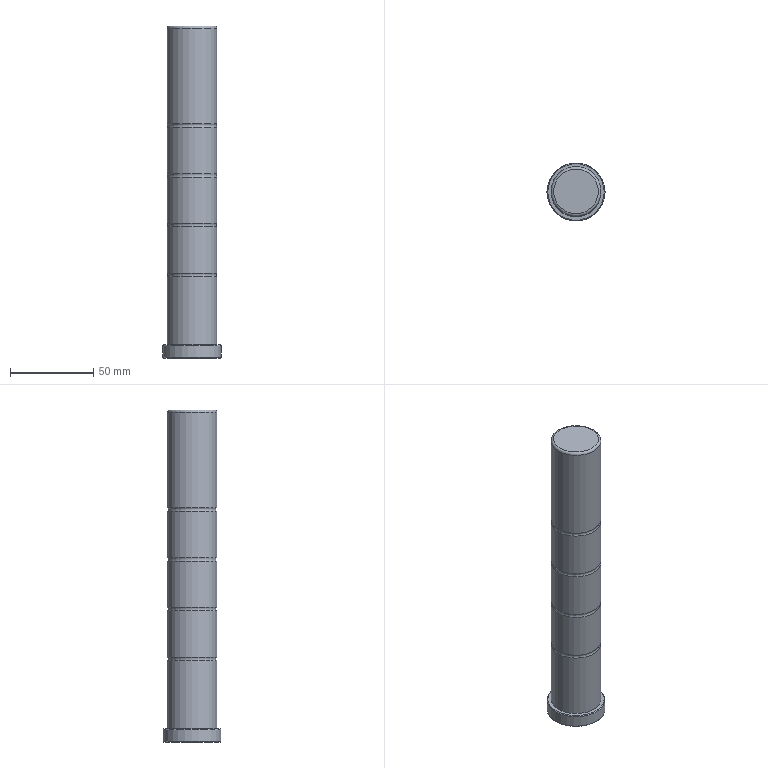Part | NX | features 模具.stp<1>[47] 2 | 1 solid | 24 faces | box 35 x 35 x 200 mm | volume 140384 mm3 | cylinder 9 | plane 7 | torus 5 | cone 3 | commonest cylinder face diameters 30 x5 10.5 x1 11.7 x1 12 x1 35 x1
STEP:
#1=CARTESIAN_POINT('',(160.,-265.,-252.505));
#2=VERTEX_POINT('',#1);
#3=VERTEX_LOOP('',#2);
#4=FACE_BOUND('',#3,.T.);
#5=CARTESIAN_POINT('',(165.25,-265.,-255.536));
#6=VERTEX_POINT('',#5);
#7=CARTESIAN_POINT('',(160.,-265.,-255.536));
#8=DIRECTION('',(0.,0.,1.));
#9=DIRECTION('',(1.,0.,0.));
#10=AXIS2_PLACEMENT_3D('',#7,#8,#9);
#11=CIRCLE('',#10,5.25);
#12=EDGE_CURVE('',#6,#6,#11,.T.);
#13=ORIENTED_EDGE('',*,*,#12,.F.);
#14=EDGE_LOOP('',(#13));
#15=FACE_BOUND('',#14,.T.);
#16=CARTESIAN_POINT('',(160.,-265.,-253.505));
#17=DIRECTION('',(0.,0.,-1.));
#18=DIRECTION('',(1.,0.,0.));
#19=AXIS2_PLACEMENT_3D('',#16,#17,#18);
#20=CONICAL_SURFACE('',#19,1.732,1.047);
#21=ADVANCED_FACE('',(#4,#15),#20,.F.);
#22=CARTESIAN_POINT('',(165.25,-265.,-261.5));
#23=VERTEX_POINT('',#22);
#24=CARTESIAN_POINT('',(165.25,-265.,-262.5));
#25=VERTEX_POINT('',#24);
#26=CARTESIAN_POINT('',(165.25,-265.,-255.536));
#27=DIRECTION('',(0.,0.,-1.));
#28=VECTOR('',#27,1000.);
#29=LINE('',#26,#28);
#30=EDGE_CURVE('',#23,#25,#29,.T.);
#31=ORIENTED_EDGE('',*,*,#30,.T.);
#32=CARTESIAN_POINT('',(160.,-270.25,-262.5));
#33=VERTEX_POINT('',#32);
#34=CARTESIAN_POINT('',(160.,-265.,-262.5));
#35=DIRECTION('',(0.,0.,1.));
#36=DIRECTION('',(0.,-1.,0.));
#37=AXIS2_PLACEMENT_3D('',#34,#35,#36);
#38=CIRCLE('',#37,5.25);
#39=EDGE_CURVE('',#25,#33,#38,.T.);
#40=ORIENTED_EDGE('',*,*,#39,.T.);
#41=CARTESIAN_POINT('',(160.,-270.25,-261.5));
#42=VERTEX_POINT('',#41);
#43=CARTESIAN_POINT('',(160.,-270.25,-255.536));
#44=DIRECTION('',(0.,0.,1.));
#45=VECTOR('',#44,1000.);
#46=LINE('',#43,#45);
#47=EDGE_CURVE('',#33,#42,#46,.T.);
#48=ORIENTED_EDGE('',*,*,#47,.T.);
#49=CARTESIAN_POINT('',(160.,-265.,-261.5));
#50=DIRECTION('',(0.,0.,1.));
#51=DIRECTION('',(0.,-1.,0.));
#52=AXIS2_PLACEMENT_3D('',#49,#50,#51);
#53=CIRCLE('',#52,5.25);
#54=EDGE_CURVE('',#23,#42,#53,.T.);
#55=ORIENTED_EDGE('',*,*,#54,.F.);
#56=EDGE_LOOP('',(#31,#40,#48,#55));
#57=FACE_BOUND('',#56,.T.);
#58=ORIENTED_EDGE('',*,*,#12,.T.);
#59=EDGE_LOOP('',(#58));
#60=FACE_BOUND('',#59,.T.);
#61=CARTESIAN_POINT('',(154.75,-265.,-285.5));
#62=VERTEX_POINT('',#61);
#63=CARTESIAN_POINT('',(160.,-265.,-285.5));
#64=DIRECTION('',(0.,0.,-1.));
#65=DIRECTION('',(-1.,0.,0.));
#66=AXIS2_PLACEMENT_3D('',#63,#64,#65);
#67=CIRCLE('',#66,5.25);
#68=EDGE_CURVE('',#62,#62,#67,.T.);
#69=ORIENTED_EDGE('',*,*,#68,.T.);
#70=EDGE_LOOP('',(#69));
#71=FACE_BOUND('',#70,.T.);
#72=CARTESIAN_POINT('',(160.,-265.,-255.536));
#73=DIRECTION('',(0.,0.,-1.));
#74=DIRECTION('',(1.,0.,0.));
#75=AXIS2_PLACEMENT_3D('',#72,#73,#74);
#76=CYLINDRICAL_SURFACE('',#75,5.25);
#77=ADVANCED_FACE('',(#57,#60,#71),#76,.F.);
#78=CARTESIAN_POINT('',(160.,-271.,-261.5));
#79=VERTEX_POINT('',#78);
#80=CARTESIAN_POINT('',(160.,-271.,-285.5));
#81=VERTEX_POINT('',#80);
#82=CARTESIAN_POINT('',(160.,-271.,-261.5));
#83=DIRECTION('',(0.,0.,-1.));
#84=VECTOR('',#83,1000.);
#85=LINE('',#82,#84);
#86=EDGE_CURVE('',#79,#81,#85,.T.);
#87=ORIENTED_EDGE('',*,*,#86,.F.);
#88=CARTESIAN_POINT('',(160.,-271.,-261.5));
#89=DIRECTION('',(0.,1.,0.));
#90=VECTOR('',#89,1000.);
#91=LINE('',#88,#90);
#92=EDGE_CURVE('',#79,#42,#91,.T.);
#93=ORIENTED_EDGE('',*,*,#92,.T.);
#94=ORIENTED_EDGE('',*,*,#47,.F.);
#95=CARTESIAN_POINT('',(160.,-270.85,-262.5));
#96=VERTEX_POINT('',#95);
#97=CARTESIAN_POINT('',(160.,-265.,-262.5));
#98=DIRECTION('',(0.,-1.,0.));
#99=VECTOR('',#98,1000.);
#100=LINE('',#97,#99);
#101=EDGE_CURVE('',#33,#96,#100,.T.);
#102=ORIENTED_EDGE('',*,*,#101,.T.);
#103=CARTESIAN_POINT('',(160.,-270.85,-285.5));
#104=VERTEX_POINT('',#103);
#105=CARTESIAN_POINT('',(160.,-270.85,-262.5));
#106=DIRECTION('',(0.,0.,-1.));
#107=VECTOR('',#106,1000.);
#108=LINE('',#105,#107);
#109=EDGE_CURVE('',#96,#104,#108,.T.);
#110=ORIENTED_EDGE('',*,*,#109,.T.);
#111=CARTESIAN_POINT('',(160.,-265.,-285.5));
#112=DIRECTION('',(0.,1.,0.));
#113=VECTOR('',#112,1000.);
#114=LINE('',#111,#113);
#115=EDGE_CURVE('',#81,#104,#114,.T.);
#116=ORIENTED_EDGE('',*,*,#115,.F.);
#117=EDGE_LOOP('',(#87,#93,#94,#102,#110,#116));
#118=FACE_BOUND('',#117,.T.);
#119=CARTESIAN_POINT('',(160.,-271.,-261.5));
#120=DIRECTION('',(-1.,0.,0.));
#121=DIRECTION('',(0.,0.,1.));
#122=AXIS2_PLACEMENT_3D('',#119,#120,#121);
#123=PLANE('',#122);
#124=ADVANCED_FACE('',(#118),#123,.T.);
#125=CARTESIAN_POINT('',(165.85,-265.,-285.5));
#126=VERTEX_POINT('',#125);
#127=CARTESIAN_POINT('',(165.85,-265.,-262.5));
#128=VERTEX_POINT('',#127);
#129=CARTESIAN_POINT('',(165.85,-265.,-262.5));
#130=DIRECTION('',(0.,0.,1.));
#131=VECTOR('',#130,1000.);
#132=LINE('',#129,#131);
#133=EDGE_CURVE('',#126,#128,#132,.T.);
#134=ORIENTED_EDGE('',*,*,#133,.T.);
#135=CARTESIAN_POINT('',(160.,-265.,-262.5));
#136=DIRECTION('',(-1.,0.,0.));
#137=VECTOR('',#136,1000.);
#138=LINE('',#135,#137);
#139=EDGE_CURVE('',#128,#25,#138,.T.);
#140=ORIENTED_EDGE('',*,*,#139,.T.);
#141=ORIENTED_EDGE('',*,*,#30,.F.);
#142=CARTESIAN_POINT('',(166.,-265.,-261.5));
#143=VERTEX_POINT('',#142);
#144=CARTESIAN_POINT('',(166.,-265.,-261.5));
#145=DIRECTION('',(1.,0.,0.));
#146=VECTOR('',#145,1000.);
#147=LINE('',#144,#146);
#148=EDGE_CURVE('',#23,#143,#147,.T.);
#149=ORIENTED_EDGE('',*,*,#148,.T.);
#150=CARTESIAN_POINT('',(166.,-265.,-285.5));
#151=VERTEX_POINT('',#150);
#152=CARTESIAN_POINT('',(166.,-265.,-261.5));
#153=DIRECTION('',(0.,0.,1.));
#154=VECTOR('',#153,1000.);
#155=LINE('',#152,#154);
#156=EDGE_CURVE('',#151,#143,#155,.T.);
#157=ORIENTED_EDGE('',*,*,#156,.F.);
#158=CARTESIAN_POINT('',(160.,-265.,-285.5));
#159=DIRECTION('',(1.,0.,0.));
#160=VECTOR('',#159,1000.);
#161=LINE('',#158,#160);
#162=EDGE_CURVE('',#126,#151,#161,.T.);
#163=ORIENTED_EDGE('',*,*,#162,.F.);
#164=EDGE_LOOP('',(#134,#140,#141,#149,#157,#163));
#165=FACE_BOUND('',#164,.T.);
#166=CARTESIAN_POINT('',(166.,-265.,-261.5));
#167=DIRECTION('',(0.,1.,0.));
#168=DIRECTION('',(0.,0.,-1.));
#169=AXIS2_PLACEMENT_3D('',#166,#167,#168);
#170=PLANE('',#169);
#171=ADVANCED_FACE('',(#165),#170,.T.);
#172=ORIENTED_EDGE('',*,*,#109,.F.);
#173=CARTESIAN_POINT('',(160.,-265.,-262.5));
#174=DIRECTION('',(0.,0.,-1.));
#175=DIRECTION('',(1.,0.,0.));
#176=AXIS2_PLACEMENT_3D('',#173,#174,#175);
#177=CIRCLE('',#176,5.85);
#178=EDGE_CURVE('',#96,#128,#177,.T.);
#179=ORIENTED_EDGE('',*,*,#178,.T.);
#180=ORIENTED_EDGE('',*,*,#133,.F.);
#181=CARTESIAN_POINT('',(160.,-265.,-285.5));
#182=DIRECTION('',(0.,0.,-1.));
#183=DIRECTION('',(-1.,0.,0.));
#184=AXIS2_PLACEMENT_3D('',#181,#182,#183);
#185=CIRCLE('',#184,5.85);
#186=EDGE_CURVE('',#104,#126,#185,.T.);
#187=ORIENTED_EDGE('',*,*,#186,.F.);
#188=EDGE_LOOP('',(#172,#179,#180,#187));
#189=FACE_BOUND('',#188,.T.);
#190=CARTESIAN_POINT('',(160.,-265.,-262.5));
#191=DIRECTION('',(0.,0.,-1.));
#192=DIRECTION('',(1.,0.,0.));
#193=AXIS2_PLACEMENT_3D('',#190,#191,#192);
#194=CYLINDRICAL_SURFACE('',#193,5.85);
#195=ADVANCED_FACE('',(#189),#194,.T.);
#196=ORIENTED_EDGE('',*,*,#139,.F.);
#197=ORIENTED_EDGE('',*,*,#178,.F.);
#198=ORIENTED_EDGE('',*,*,#101,.F.);
#199=ORIENTED_EDGE('',*,*,#39,.F.);
#200=EDGE_LOOP('',(#196,#197,#198,#199));
#201=FACE_BOUND('',#200,.T.);
#202=CARTESIAN_POINT('',(160.,-265.,-262.5));
#203=DIRECTION('',(0.,0.,1.));
#204=DIRECTION('',(0.,-1.,0.));
#205=AXIS2_PLACEMENT_3D('',#202,#203,#204);
#206=PLANE('',#205);
#207=ADVANCED_FACE('',(#201),#206,.T.);
#208=CARTESIAN_POINT('',(160.,-265.,-285.5));
#209=DIRECTION('',(0.,0.,-1.));
#210=DIRECTION('',(-1.,0.,0.));
#211=AXIS2_PLACEMENT_3D('',#208,#209,#210);
#212=CIRCLE('',#211,6.);
#213=EDGE_CURVE('',#81,#151,#212,.T.);
#214=ORIENTED_EDGE('',*,*,#213,.T.);
#215=ORIENTED_EDGE('',*,*,#156,.T.);
#216=CARTESIAN_POINT('',(160.,-265.,-261.5));
#217=DIRECTION('',(0.,0.,-1.));
#218=DIRECTION('',(1.,0.,0.));
#219=AXIS2_PLACEMENT_3D('',#216,#217,#218);
#220=CIRCLE('',#219,6.);
#221=EDGE_CURVE('',#79,#143,#220,.T.);
#222=ORIENTED_EDGE('',*,*,#221,.F.);
#223=ORIENTED_EDGE('',*,*,#86,.T.);
#224=EDGE_LOOP('',(#214,#215,#222,#223));
#225=FACE_BOUND('',#224,.T.);
#226=CARTESIAN_POINT('',(160.,-265.,-261.5));
#227=DIRECTION('',(0.,0.,-1.));
#228=DIRECTION('',(1.,0.,0.));
#229=AXIS2_PLACEMENT_3D('',#226,#227,#228);
#230=CYLINDRICAL_SURFACE('',#229,6.);
#231=ADVANCED_FACE('',(#225),#230,.F.);
#232=ORIENTED_EDGE('',*,*,#54,.T.);
#233=ORIENTED_EDGE('',*,*,#92,.F.);
#234=ORIENTED_EDGE('',*,*,#221,.T.);
#235=ORIENTED_EDGE('',*,*,#148,.F.);
#236=EDGE_LOOP('',(#232,#233,#234,#235));
#237=FACE_BOUND('',#236,.T.);
#238=CARTESIAN_POINT('',(160.,-265.,-261.5));
#239=DIRECTION('',(0.,0.,1.));
#240=DIRECTION('',(0.,-1.,0.));
#241=AXIS2_PLACEMENT_3D('',#238,#239,#240);
#242=PLANE('',#241);
#243=ADVANCED_FACE('',(#237),#242,.F.);
#244=CARTESIAN_POINT('',(175.,-265.,-87.));
#245=VERTEX_POINT('',#244);
#246=CARTESIAN_POINT('',(160.,-265.,-87.));
#247=DIRECTION('',(0.,0.,-1.));
#248=DIRECTION('',(1.,0.,0.));
#249=AXIS2_PLACEMENT_3D('',#246,#247,#248);
#250=CIRCLE('',#249,15.);
#251=EDGE_CURVE('',#245,#245,#250,.T.);
#252=ORIENTED_EDGE('',*,*,#251,.T.);
#253=EDGE_LOOP('',(#252));
#254=FACE_BOUND('',#253,.T.);
#255=CARTESIAN_POINT('',(145.,-265.,-144.446));
#256=VERTEX_POINT('',#255);
#257=CARTESIAN_POINT('',(160.,-265.,-144.446));
#258=DIRECTION('',(0.,0.,-1.));
#259=DIRECTION('',(-1.,0.,0.));
#260=AXIS2_PLACEMENT_3D('',#257,#258,#259);
#261=CIRCLE('',#260,15.);
#262=EDGE_CURVE('',#256,#256,#261,.T.);
#263=ORIENTED_EDGE('',*,*,#262,.F.);
#264=EDGE_LOOP('',(#263));
#265=FACE_BOUND('',#264,.T.);
#266=CARTESIAN_POINT('',(160.,-265.,-285.5));
#267=DIRECTION('',(0.,0.,1.));
#268=DIRECTION('',(1.,0.,0.));
#269=AXIS2_PLACEMENT_3D('',#266,#267,#268);
#270=CYLINDRICAL_SURFACE('',#269,15.);
#271=ADVANCED_FACE('',(#254,#265),#270,.T.);
#272=ORIENTED_EDGE('',*,*,#251,.F.);
#273=EDGE_LOOP('',(#272));
#274=FACE_BOUND('',#273,.T.);
#275=CARTESIAN_POINT('',(173.5,-265.,-85.5));
#276=VERTEX_POINT('',#275);
#277=CARTESIAN_POINT('',(160.,-265.,-85.5));
#278=DIRECTION('',(0.,0.,1.));
#279=DIRECTION('',(1.,0.,0.));
#280=AXIS2_PLACEMENT_3D('',#277,#278,#279);
#281=CIRCLE('',#280,13.5);
#282=EDGE_CURVE('',#276,#276,#281,.T.);
#283=ORIENTED_EDGE('',*,*,#282,.F.);
#284=EDGE_LOOP('',(#283));
#285=FACE_BOUND('',#284,.T.);
#286=CARTESIAN_POINT('',(160.,-265.,-87.));
#287=DIRECTION('',(0.,0.,1.));
#288=DIRECTION('',(1.,0.,0.));
#289=AXIS2_PLACEMENT_3D('',#286,#287,#288);
#290=TOROIDAL_SURFACE('',#289,13.5,1.5);
#291=ADVANCED_FACE('',(#274,#285),#290,.T.);
#292=ORIENTED_EDGE('',*,*,#282,.T.);
#293=EDGE_LOOP('',(#292));
#294=FACE_BOUND('',#293,.T.);
#295=CARTESIAN_POINT('',(160.,-265.,-85.5));
#296=DIRECTION('',(0.,0.,1.));
#297=DIRECTION('',(1.,0.,0.));
#298=AXIS2_PLACEMENT_3D('',#295,#296,#297);
#299=PLANE('',#298);
#300=ADVANCED_FACE('',(#294),#299,.T.);
#301=CARTESIAN_POINT('',(175.,-265.,-146.554));
#302=VERTEX_POINT('',#301);
#303=CARTESIAN_POINT('',(160.,-265.,-146.554));
#304=DIRECTION('',(0.,0.,1.));
#305=DIRECTION('',(1.,0.,0.));
#306=AXIS2_PLACEMENT_3D('',#303,#304,#305);
#307=CIRCLE('',#306,15.);
#308=EDGE_CURVE('',#302,#302,#307,.T.);
#309=ORIENTED_EDGE('',*,*,#308,.T.);
#310=EDGE_LOOP('',(#309));
#311=FACE_BOUND('',#310,.T.);
#312=ORIENTED_EDGE('',*,*,#262,.T.);
#313=EDGE_LOOP('',(#312));
#314=FACE_BOUND('',#313,.T.);
#315=CARTESIAN_POINT('',(160.,-265.,-145.5));
#316=DIRECTION('',(0.,0.,1.));
#317=DIRECTION('',(1.,0.,0.));
#318=AXIS2_PLACEMENT_3D('',#315,#316,#317);
#319=TOROIDAL_SURFACE('',#318,16.7,2.);
#320=ADVANCED_FACE('',(#311,#314),#319,.F.);
#321=ORIENTED_EDGE('',*,*,#308,.F.);
#322=EDGE_LOOP('',(#321));
#323=FACE_BOUND('',#322,.T.);
#324=CARTESIAN_POINT('',(145.,-265.,-174.446));
#325=VERTEX_POINT('',#324);
#326=CARTESIAN_POINT('',(160.,-265.,-174.446));
#327=DIRECTION('',(0.,0.,-1.));
#328=DIRECTION('',(-1.,0.,0.));
#329=AXIS2_PLACEMENT_3D('',#326,#327,#328);
#330=CIRCLE('',#329,15.);
#331=EDGE_CURVE('',#325,#325,#330,.T.);
#332=ORIENTED_EDGE('',*,*,#331,.F.);
#333=EDGE_LOOP('',(#332));
#334=FACE_BOUND('',#333,.T.);
#335=CARTESIAN_POINT('',(160.,-265.,-285.5));
#336=DIRECTION('',(0.,0.,1.));
#337=DIRECTION('',(1.,0.,0.));
#338=AXIS2_PLACEMENT_3D('',#335,#336,#337);
#339=CYLINDRICAL_SURFACE('',#338,15.);
#340=ADVANCED_FACE('',(#323,#334),#339,.T.);
#341=CARTESIAN_POINT('',(175.,-265.,-176.554));
#342=VERTEX_POINT('',#341);
#343=CARTESIAN_POINT('',(160.,-265.,-176.554));
#344=DIRECTION('',(0.,0.,1.));
#345=DIRECTION('',(1.,0.,0.));
#346=AXIS2_PLACEMENT_3D('',#343,#344,#345);
#347=CIRCLE('',#346,15.);
#348=EDGE_CURVE('',#342,#342,#347,.T.);
#349=ORIENTED_EDGE('',*,*,#348,.T.);
#350=EDGE_LOOP('',(#349));
#351=FACE_BOUND('',#350,.T.);
#352=ORIENTED_EDGE('',*,*,#331,.T.);
#353=EDGE_LOOP('',(#352));
#354=FACE_BOUND('',#353,.T.);
#355=CARTESIAN_POINT('',(160.,-265.,-175.5));
#356=DIRECTION('',(0.,0.,1.));
#357=DIRECTION('',(1.,0.,0.));
#358=AXIS2_PLACEMENT_3D('',#355,#356,#357);
#359=TOROIDAL_SURFACE('',#358,16.7,2.);
#360=ADVANCED_FACE('',(#351,#354),#359,.F.);
#361=ORIENTED_EDGE('',*,*,#348,.F.);
#362=EDGE_LOOP('',(#361));
#363=FACE_BOUND('',#362,.T.);
#364=CARTESIAN_POINT('',(145.,-265.,-204.446));
#365=VERTEX_POINT('',#364);
#366=CARTESIAN_POINT('',(160.,-265.,-204.446));
#367=DIRECTION('',(0.,0.,-1.));
#368=DIRECTION('',(-1.,0.,0.));
#369=AXIS2_PLACEMENT_3D('',#366,#367,#368);
#370=CIRCLE('',#369,15.);
#371=EDGE_CURVE('',#365,#365,#370,.T.);
#372=ORIENTED_EDGE('',*,*,#371,.F.);
#373=EDGE_LOOP('',(#372));
#374=FACE_BOUND('',#373,.T.);
#375=CARTESIAN_POINT('',(160.,-265.,-285.5));
#376=DIRECTION('',(0.,0.,1.));
#377=DIRECTION('',(1.,0.,0.));
#378=AXIS2_PLACEMENT_3D('',#375,#376,#377);
#379=CYLINDRICAL_SURFACE('',#378,15.);
#380=ADVANCED_FACE('',(#363,#374),#379,.T.);
#381=CARTESIAN_POINT('',(175.,-265.,-206.554));
#382=VERTEX_POINT('',#381);
#383=CARTESIAN_POINT('',(160.,-265.,-206.554));
#384=DIRECTION('',(0.,0.,1.));
#385=DIRECTION('',(1.,0.,0.));
#386=AXIS2_PLACEMENT_3D('',#383,#384,#385);
#387=CIRCLE('',#386,15.);
#388=EDGE_CURVE('',#382,#382,#387,.T.);
#389=ORIENTED_EDGE('',*,*,#388,.T.);
#390=EDGE_LOOP('',(#389));
#391=FACE_BOUND('',#390,.T.);
#392=ORIENTED_EDGE('',*,*,#371,.T.);
#393=EDGE_LOOP('',(#392));
#394=FACE_BOUND('',#393,.T.);
#395=CARTESIAN_POINT('',(160.,-265.,-205.5));
#396=DIRECTION('',(0.,0.,1.));
#397=DIRECTION('',(1.,0.,0.));
#398=AXIS2_PLACEMENT_3D('',#395,#396,#397);
#399=TOROIDAL_SURFACE('',#398,16.7,2.);
#400=ADVANCED_FACE('',(#391,#394),#399,.F.);
#401=ORIENTED_EDGE('',*,*,#388,.F.);
#402=EDGE_LOOP('',(#401));
#403=FACE_BOUND('',#402,.T.);
#404=CARTESIAN_POINT('',(145.,-265.,-234.446));
#405=VERTEX_POINT('',#404);
#406=CARTESIAN_POINT('',(160.,-265.,-234.446));
#407=DIRECTION('',(0.,0.,-1.));
#408=DIRECTION('',(-1.,0.,0.));
#409=AXIS2_PLACEMENT_3D('',#406,#407,#408);
#410=CIRCLE('',#409,15.);
#411=EDGE_CURVE('',#405,#405,#410,.T.);
#412=ORIENTED_EDGE('',*,*,#411,.F.);
#413=EDGE_LOOP('',(#412));
#414=FACE_BOUND('',#413,.T.);
#415=CARTESIAN_POINT('',(160.,-265.,-285.5));
#416=DIRECTION('',(0.,0.,1.));
#417=DIRECTION('',(1.,0.,0.));
#418=AXIS2_PLACEMENT_3D('',#415,#416,#417);
#419=CYLINDRICAL_SURFACE('',#418,15.);
#420=ADVANCED_FACE('',(#403,#414),#419,.T.);
#421=CARTESIAN_POINT('',(175.,-265.,-236.554));
#422=VERTEX_POINT('',#421);
#423=CARTESIAN_POINT('',(160.,-265.,-236.554));
#424=DIRECTION('',(0.,0.,1.));
#425=DIRECTION('',(1.,0.,0.));
#426=AXIS2_PLACEMENT_3D('',#423,#424,#425);
#427=CIRCLE('',#426,15.);
#428=EDGE_CURVE('',#422,#422,#427,.T.);
#429=ORIENTED_EDGE('',*,*,#428,.T.);
#430=EDGE_LOOP('',(#429));
#431=FACE_BOUND('',#430,.T.);
#432=ORIENTED_EDGE('',*,*,#411,.T.);
#433=EDGE_LOOP('',(#432));
#434=FACE_BOUND('',#433,.T.);
#435=CARTESIAN_POINT('',(160.,-265.,-235.5));
#436=DIRECTION('',(0.,0.,1.));
#437=DIRECTION('',(1.,0.,0.));
#438=AXIS2_PLACEMENT_3D('',#435,#436,#437);
#439=TOROIDAL_SURFACE('',#438,16.7,2.);
#440=ADVANCED_FACE('',(#431,#434),#439,.F.);
#441=CARTESIAN_POINT('',(175.,-265.,-277.5));
#442=VERTEX_POINT('',#441);
#443=CARTESIAN_POINT('',(160.,-265.,-277.5));
#444=DIRECTION('',(0.,0.,1.));
#445=DIRECTION('',(1.,0.,0.));
#446=AXIS2_PLACEMENT_3D('',#443,#444,#445);
#447=CIRCLE('',#446,15.);
#448=EDGE_CURVE('',#442,#442,#447,.T.);
#449=ORIENTED_EDGE('',*,*,#448,.T.);
#450=EDGE_LOOP('',(#449));
#451=FACE_BOUND('',#450,.T.);
#452=ORIENTED_EDGE('',*,*,#428,.F.);
#453=EDGE_LOOP('',(#452));
#454=FACE_BOUND('',#453,.T.);
#455=CARTESIAN_POINT('',(160.,-265.,-285.5));
#456=DIRECTION('',(0.,0.,1.));
#457=DIRECTION('',(1.,0.,0.));
#458=AXIS2_PLACEMENT_3D('',#455,#456,#457);
#459=CYLINDRICAL_SURFACE('',#458,15.);
#460=ADVANCED_FACE('',(#451,#454),#459,.T.);
#461=CARTESIAN_POINT('',(177.5,-265.,-278.));
#462=VERTEX_POINT('',#461);
#463=CARTESIAN_POINT('',(160.,-265.,-278.));
#464=DIRECTION('',(0.,0.,-1.));
#465=DIRECTION('',(1.,0.,0.));
#466=AXIS2_PLACEMENT_3D('',#463,#464,#465);
#467=CIRCLE('',#466,17.5);
#468=EDGE_CURVE('',#462,#462,#467,.T.);
#469=ORIENTED_EDGE('',*,*,#468,.F.);
#470=EDGE_LOOP('',(#469));
#471=FACE_BOUND('',#470,.T.);
#472=CARTESIAN_POINT('',(177.,-265.,-277.5));
#473=VERTEX_POINT('',#472);
#474=CARTESIAN_POINT('',(160.,-265.,-277.5));
#475=DIRECTION('',(0.,0.,1.));
#476=DIRECTION('',(1.,0.,0.));
#477=AXIS2_PLACEMENT_3D('',#474,#475,#476);
#478=CIRCLE('',#477,17.);
#479=EDGE_CURVE('',#473,#473,#478,.T.);
#480=ORIENTED_EDGE('',*,*,#479,.F.);
#481=EDGE_LOOP('',(#480));
#482=FACE_BOUND('',#481,.T.);
#483=CARTESIAN_POINT('',(160.,-265.,-278.));
#484=DIRECTION('',(0.,0.,-1.));
#485=DIRECTION('',(-1.,0.,0.));
#486=AXIS2_PLACEMENT_3D('',#483,#484,#485);
#487=CONICAL_SURFACE('',#486,17.5,0.7854);
#488=ADVANCED_FACE('',(#471,#482),#487,.T.);
#489=CARTESIAN_POINT('',(142.5,-265.,-285.));
#490=VERTEX_POINT('',#489);
#491=CARTESIAN_POINT('',(160.,-265.,-285.));
#492=DIRECTION('',(0.,0.,1.));
#493=DIRECTION('',(-1.,0.,0.));
#494=AXIS2_PLACEMENT_3D('',#491,#492,#493);
#495=CIRCLE('',#494,17.5);
#496=EDGE_CURVE('',#490,#490,#495,.T.);
#497=ORIENTED_EDGE('',*,*,#496,.F.);
#498=EDGE_LOOP('',(#497));
#499=FACE_BOUND('',#498,.T.);
#500=CARTESIAN_POINT('',(143.,-265.,-285.5));
#501=VERTEX_POINT('',#500);
#502=CARTESIAN_POINT('',(160.,-265.,-285.5));
#503=DIRECTION('',(0.,0.,-1.));
#504=DIRECTION('',(-1.,0.,0.));
#505=AXIS2_PLACEMENT_3D('',#502,#503,#504);
#506=CIRCLE('',#505,17.);
#507=EDGE_CURVE('',#501,#501,#506,.T.);
#508=ORIENTED_EDGE('',*,*,#507,.F.);
#509=EDGE_LOOP('',(#508));
#510=FACE_BOUND('',#509,.T.);
#511=CARTESIAN_POINT('',(160.,-265.,-285.));
#512=DIRECTION('',(0.,0.,1.));
#513=DIRECTION('',(1.,0.,0.));
#514=AXIS2_PLACEMENT_3D('',#511,#512,#513);
#515=CONICAL_SURFACE('',#514,17.5,0.7854);
#516=ADVANCED_FACE('',(#499,#510),#515,.T.);
#517=ORIENTED_EDGE('',*,*,#468,.T.);
#518=EDGE_LOOP('',(#517));
#519=FACE_BOUND('',#518,.T.);
#520=ORIENTED_EDGE('',*,*,#496,.T.);
#521=EDGE_LOOP('',(#520));
#522=FACE_BOUND('',#521,.T.);
#523=CARTESIAN_POINT('',(160.,-265.,-285.5));
#524=DIRECTION('',(0.,0.,1.));
#525=DIRECTION('',(1.,0.,0.));
#526=AXIS2_PLACEMENT_3D('',#523,#524,#525);
#527=CYLINDRICAL_SURFACE('',#526,17.5);
#528=ADVANCED_FACE('',(#519,#522),#527,.T.);
#529=ORIENTED_EDGE('',*,*,#186,.T.);
#530=ORIENTED_EDGE('',*,*,#162,.T.);
#531=ORIENTED_EDGE('',*,*,#213,.F.);
#532=ORIENTED_EDGE('',*,*,#115,.T.);
#533=EDGE_LOOP('',(#529,#530,#531,#532));
#534=FACE_BOUND('',#533,.T.);
#535=ORIENTED_EDGE('',*,*,#68,.F.);
#536=EDGE_LOOP('',(#535));
#537=FACE_BOUND('',#536,.T.);
#538=ORIENTED_EDGE('',*,*,#507,.T.);
#539=EDGE_LOOP('',(#538));
#540=FACE_BOUND('',#539,.T.);
#541=CARTESIAN_POINT('',(160.,-265.,-285.5));
#542=DIRECTION('',(0.,0.,-1.));
#543=DIRECTION('',(0.,-1.,0.));
#544=AXIS2_PLACEMENT_3D('',#541,#542,#543);
#545=PLANE('',#544);
#546=ADVANCED_FACE('',(#534,#537,#540),#545,.T.);
#547=ORIENTED_EDGE('',*,*,#479,.T.);
#548=EDGE_LOOP('',(#547));
#549=FACE_BOUND('',#548,.T.);
#550=ORIENTED_EDGE('',*,*,#448,.F.);
#551=EDGE_LOOP('',(#550));
#552=FACE_BOUND('',#551,.T.);
#553=CARTESIAN_POINT('',(160.,-265.,-277.5));
#554=DIRECTION('',(0.,0.,1.));
#555=DIRECTION('',(1.,0.,0.));
#556=AXIS2_PLACEMENT_3D('',#553,#554,#555);
#557=PLANE('',#556);
#558=ADVANCED_FACE('',(#549,#552),#557,.T.);
#559=CLOSED_SHELL('',(#21,#77,#124,#171,#195,#207,#231,#243,#271,#291,#300,#320,#340,#360,#380,#400,#420,#440,#460,#488,#516,#528,#546,#558));
#560=MANIFOLD_SOLID_BREP('',#559);
#561=(LENGTH_UNIT()NAMED_UNIT(*)SI_UNIT(.MILLI.,.METRE.));
#562=UNCERTAINTY_MEASURE_WITH_UNIT(LENGTH_MEASURE(0.00001),#561,'','');
#563=(NAMED_UNIT(*)PLANE_ANGLE_UNIT()SI_UNIT($,.RADIAN.));
#564=(NAMED_UNIT(*)SI_UNIT($,.STERADIAN.)SOLID_ANGLE_UNIT());
#565=(GEOMETRIC_REPRESENTATION_CONTEXT(3)GLOBAL_UNCERTAINTY_ASSIGNED_CONTEXT((#562))GLOBAL_UNIT_ASSIGNED_CONTEXT((#561,#563,#564))REPRESENTATION_CONTEXT('',''));
#566=ADVANCED_BREP_SHAPE_REPRESENTATION('',(#560),#565);